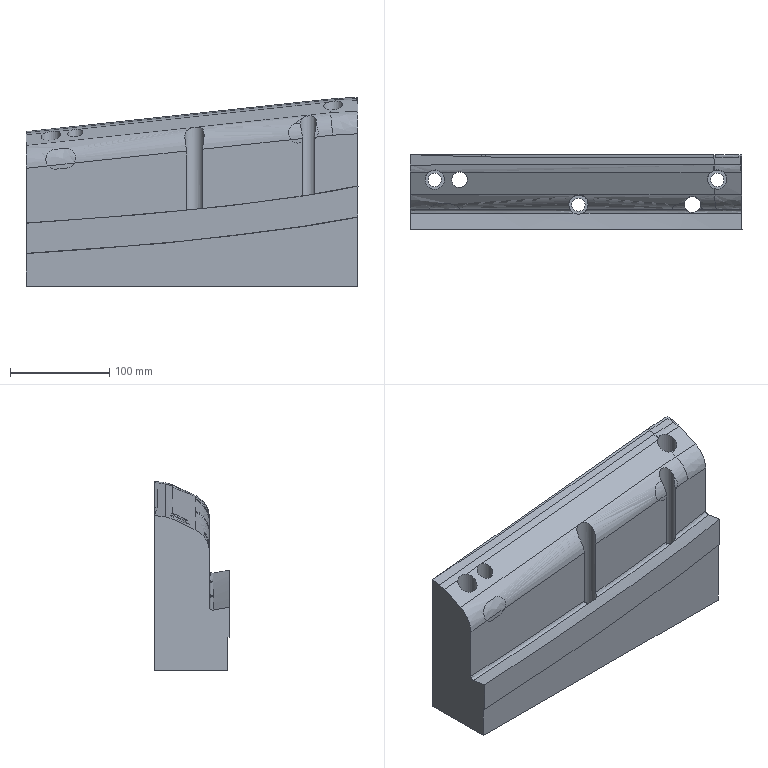Part | NX | features solid 2 | 1 solid | 49 faces | box 335 x 74.869 x 190.433 mm | volume 3317450 mm3 | spline 34 | cylinder 8 | plane 7 | commonest cylinder face diameters 13.5 x3 19.5 x3 16 x2